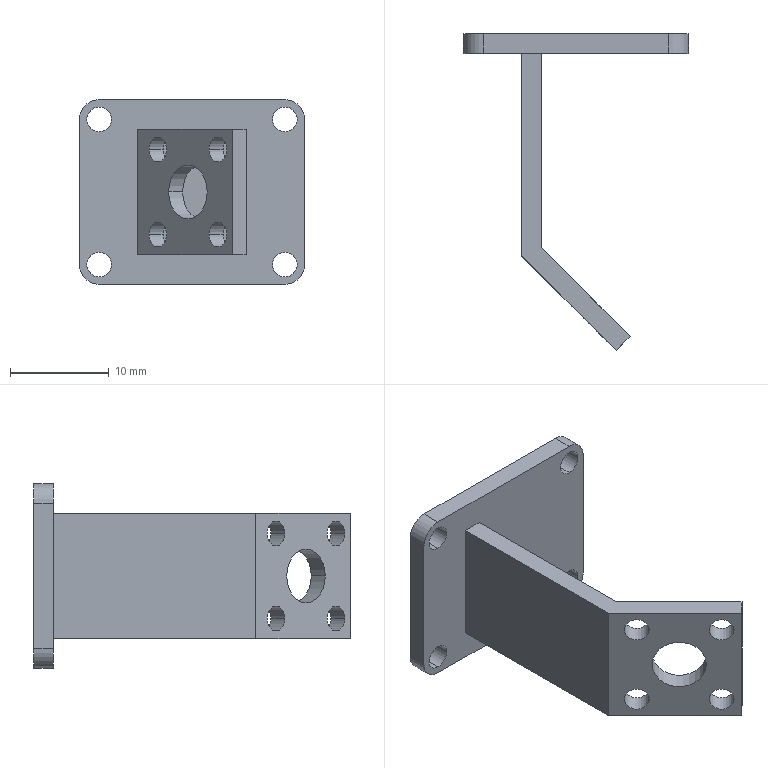Part | SolidWorks | features ICE 4, ExtruThin 1, Fillet 1 | 2 solids | 36 faces | box 22.8 x 32.073 x 18.7 mm | volume 1563 mm3 | cylinder 22 | plane 14 | commonest cylinder face diameters 2.5 x16 4 x4 5.5 x2
STEP:
#1=CARTESIAN_POINT('',(36.275,113.634,-14.95));
#2=VERTEX_POINT('',#1);
#3=CARTESIAN_POINT('',(36.275,113.634,-12.45));
#4=VERTEX_POINT('',#3);
#5=CARTESIAN_POINT('',(36.275,113.634,-13.7));
#6=DIRECTION('',(0.,1.,0.));
#7=DIRECTION('',(0.,0.,1.));
#8=AXIS2_PLACEMENT_3D('',#5,#6,#7);
#9=CIRCLE('',#8,1.25);
#10=EDGE_CURVE('',#2,#4,#9,.T.);
#11=ORIENTED_EDGE('',*,*,#10,.F.);
#12=CARTESIAN_POINT('',(36.275,115.634,-14.95));
#13=VERTEX_POINT('',#12);
#14=CARTESIAN_POINT('',(36.275,113.634,-14.95));
#15=DIRECTION('',(0.,1.,0.));
#16=VECTOR('',#15,1000.);
#17=LINE('',#14,#16);
#18=EDGE_CURVE('',#2,#13,#17,.T.);
#19=ORIENTED_EDGE('',*,*,#18,.T.);
#20=CARTESIAN_POINT('',(36.275,115.634,-12.45));
#21=VERTEX_POINT('',#20);
#22=CARTESIAN_POINT('',(36.275,115.634,-13.7));
#23=DIRECTION('',(0.,1.,0.));
#24=DIRECTION('',(0.,0.,1.));
#25=AXIS2_PLACEMENT_3D('',#22,#23,#24);
#26=CIRCLE('',#25,1.25);
#27=EDGE_CURVE('',#13,#21,#26,.T.);
#28=ORIENTED_EDGE('',*,*,#27,.T.);
#29=CARTESIAN_POINT('',(36.275,113.634,-12.45));
#30=DIRECTION('',(0.,1.,0.));
#31=VECTOR('',#30,1000.);
#32=LINE('',#29,#31);
#33=EDGE_CURVE('',#4,#21,#32,.T.);
#34=ORIENTED_EDGE('',*,*,#33,.F.);
#35=EDGE_LOOP('',(#11,#19,#28,#34));
#36=FACE_OUTER_BOUND('',#35,.T.);
#37=CARTESIAN_POINT('',(36.275,113.634,-13.7));
#38=DIRECTION('',(0.,1.,0.));
#39=DIRECTION('',(0.,0.,1.));
#40=AXIS2_PLACEMENT_3D('',#37,#38,#39);
#41=CYLINDRICAL_SURFACE('',#40,1.25);
#42=ADVANCED_FACE('',(#36),#41,.F.);
#43=CARTESIAN_POINT('',(36.275,113.634,-0.25));
#44=VERTEX_POINT('',#43);
#45=CARTESIAN_POINT('',(36.275,113.634,2.25));
#46=VERTEX_POINT('',#45);
#47=CARTESIAN_POINT('',(36.275,113.634,1.));
#48=DIRECTION('',(0.,1.,0.));
#49=DIRECTION('',(0.,0.,1.));
#50=AXIS2_PLACEMENT_3D('',#47,#48,#49);
#51=CIRCLE('',#50,1.25);
#52=EDGE_CURVE('',#44,#46,#51,.T.);
#53=ORIENTED_EDGE('',*,*,#52,.F.);
#54=CARTESIAN_POINT('',(36.275,115.634,-0.25));
#55=VERTEX_POINT('',#54);
#56=CARTESIAN_POINT('',(36.275,113.634,-0.25));
#57=DIRECTION('',(0.,1.,0.));
#58=VECTOR('',#57,1000.);
#59=LINE('',#56,#58);
#60=EDGE_CURVE('',#44,#55,#59,.T.);
#61=ORIENTED_EDGE('',*,*,#60,.T.);
#62=CARTESIAN_POINT('',(36.275,115.634,2.25));
#63=VERTEX_POINT('',#62);
#64=CARTESIAN_POINT('',(36.275,115.634,1.));
#65=DIRECTION('',(0.,1.,0.));
#66=DIRECTION('',(0.,0.,1.));
#67=AXIS2_PLACEMENT_3D('',#64,#65,#66);
#68=CIRCLE('',#67,1.25);
#69=EDGE_CURVE('',#55,#63,#68,.T.);
#70=ORIENTED_EDGE('',*,*,#69,.T.);
#71=CARTESIAN_POINT('',(36.275,113.634,2.25));
#72=DIRECTION('',(0.,1.,0.));
#73=VECTOR('',#72,1000.);
#74=LINE('',#71,#73);
#75=EDGE_CURVE('',#46,#63,#74,.T.);
#76=ORIENTED_EDGE('',*,*,#75,.F.);
#77=EDGE_LOOP('',(#53,#61,#70,#76));
#78=FACE_OUTER_BOUND('',#77,.T.);
#79=CARTESIAN_POINT('',(36.275,113.634,1.));
#80=DIRECTION('',(0.,1.,0.));
#81=DIRECTION('',(0.,0.,1.));
#82=AXIS2_PLACEMENT_3D('',#79,#80,#81);
#83=CYLINDRICAL_SURFACE('',#82,1.25);
#84=ADVANCED_FACE('',(#78),#83,.F.);
#85=CARTESIAN_POINT('',(55.075,113.634,-0.25));
#86=VERTEX_POINT('',#85);
#87=CARTESIAN_POINT('',(55.075,113.634,2.25));
#88=VERTEX_POINT('',#87);
#89=CARTESIAN_POINT('',(55.075,113.634,1.));
#90=DIRECTION('',(0.,1.,0.));
#91=DIRECTION('',(0.,0.,1.));
#92=AXIS2_PLACEMENT_3D('',#89,#90,#91);
#93=CIRCLE('',#92,1.25);
#94=EDGE_CURVE('',#86,#88,#93,.T.);
#95=ORIENTED_EDGE('',*,*,#94,.F.);
#96=CARTESIAN_POINT('',(55.075,115.634,-0.25));
#97=VERTEX_POINT('',#96);
#98=CARTESIAN_POINT('',(55.075,113.634,-0.25));
#99=DIRECTION('',(0.,1.,0.));
#100=VECTOR('',#99,1000.);
#101=LINE('',#98,#100);
#102=EDGE_CURVE('',#86,#97,#101,.T.);
#103=ORIENTED_EDGE('',*,*,#102,.T.);
#104=CARTESIAN_POINT('',(55.075,115.634,2.25));
#105=VERTEX_POINT('',#104);
#106=CARTESIAN_POINT('',(55.075,115.634,1.));
#107=DIRECTION('',(0.,1.,0.));
#108=DIRECTION('',(0.,0.,1.));
#109=AXIS2_PLACEMENT_3D('',#106,#107,#108);
#110=CIRCLE('',#109,1.25);
#111=EDGE_CURVE('',#97,#105,#110,.T.);
#112=ORIENTED_EDGE('',*,*,#111,.T.);
#113=CARTESIAN_POINT('',(55.075,113.634,2.25));
#114=DIRECTION('',(0.,1.,0.));
#115=VECTOR('',#114,1000.);
#116=LINE('',#113,#115);
#117=EDGE_CURVE('',#88,#105,#116,.T.);
#118=ORIENTED_EDGE('',*,*,#117,.F.);
#119=EDGE_LOOP('',(#95,#103,#112,#118));
#120=FACE_OUTER_BOUND('',#119,.T.);
#121=CARTESIAN_POINT('',(55.075,113.634,1.));
#122=DIRECTION('',(0.,1.,0.));
#123=DIRECTION('',(0.,0.,1.));
#124=AXIS2_PLACEMENT_3D('',#121,#122,#123);
#125=CYLINDRICAL_SURFACE('',#124,1.25);
#126=ADVANCED_FACE('',(#120),#125,.F.);
#127=CARTESIAN_POINT('',(55.075,113.634,-14.95));
#128=VERTEX_POINT('',#127);
#129=CARTESIAN_POINT('',(55.075,113.634,-12.45));
#130=VERTEX_POINT('',#129);
#131=CARTESIAN_POINT('',(55.075,113.634,-13.7));
#132=DIRECTION('',(0.,1.,0.));
#133=DIRECTION('',(0.,0.,1.));
#134=AXIS2_PLACEMENT_3D('',#131,#132,#133);
#135=CIRCLE('',#134,1.25);
#136=EDGE_CURVE('',#128,#130,#135,.T.);
#137=ORIENTED_EDGE('',*,*,#136,.F.);
#138=CARTESIAN_POINT('',(55.075,115.634,-14.95));
#139=VERTEX_POINT('',#138);
#140=CARTESIAN_POINT('',(55.075,113.634,-14.95));
#141=DIRECTION('',(0.,1.,0.));
#142=VECTOR('',#141,1000.);
#143=LINE('',#140,#142);
#144=EDGE_CURVE('',#128,#139,#143,.T.);
#145=ORIENTED_EDGE('',*,*,#144,.T.);
#146=CARTESIAN_POINT('',(55.075,115.634,-12.45));
#147=VERTEX_POINT('',#146);
#148=CARTESIAN_POINT('',(55.075,115.634,-13.7));
#149=DIRECTION('',(0.,1.,0.));
#150=DIRECTION('',(0.,0.,1.));
#151=AXIS2_PLACEMENT_3D('',#148,#149,#150);
#152=CIRCLE('',#151,1.25);
#153=EDGE_CURVE('',#139,#147,#152,.T.);
#154=ORIENTED_EDGE('',*,*,#153,.T.);
#155=CARTESIAN_POINT('',(55.075,113.634,-12.45));
#156=DIRECTION('',(0.,1.,0.));
#157=VECTOR('',#156,1000.);
#158=LINE('',#155,#157);
#159=EDGE_CURVE('',#130,#147,#158,.T.);
#160=ORIENTED_EDGE('',*,*,#159,.F.);
#161=EDGE_LOOP('',(#137,#145,#154,#160));
#162=FACE_OUTER_BOUND('',#161,.T.);
#163=CARTESIAN_POINT('',(55.075,113.634,-13.7));
#164=DIRECTION('',(0.,1.,0.));
#165=DIRECTION('',(0.,0.,1.));
#166=AXIS2_PLACEMENT_3D('',#163,#164,#165);
#167=CYLINDRICAL_SURFACE('',#166,1.25);
#168=ADVANCED_FACE('',(#162),#167,.F.);
#169=CARTESIAN_POINT('',(57.075,115.634,1.));
#170=VERTEX_POINT('',#169);
#171=CARTESIAN_POINT('',(57.075,115.634,-13.7));
#172=VERTEX_POINT('',#171);
#173=CARTESIAN_POINT('',(57.075,115.634,-15.7));
#174=DIRECTION('',(0.,0.,-1.));
#175=VECTOR('',#174,1000.);
#176=LINE('',#173,#175);
#177=EDGE_CURVE('',#170,#172,#176,.T.);
#178=ORIENTED_EDGE('',*,*,#177,.F.);
#179=CARTESIAN_POINT('',(57.075,113.634,1.));
#180=VERTEX_POINT('',#179);
#181=CARTESIAN_POINT('',(57.075,115.634,1.));
#182=DIRECTION('',(0.,-1.,0.));
#183=VECTOR('',#182,1000.);
#184=LINE('',#181,#183);
#185=EDGE_CURVE('',#170,#180,#184,.T.);
#186=ORIENTED_EDGE('',*,*,#185,.T.);
#187=CARTESIAN_POINT('',(57.075,113.634,-13.7));
#188=VERTEX_POINT('',#187);
#189=CARTESIAN_POINT('',(57.075,113.634,-15.7));
#190=DIRECTION('',(0.,0.,-1.));
#191=VECTOR('',#190,1000.);
#192=LINE('',#189,#191);
#193=EDGE_CURVE('',#180,#188,#192,.T.);
#194=ORIENTED_EDGE('',*,*,#193,.T.);
#195=CARTESIAN_POINT('',(57.075,115.634,-13.7));
#196=DIRECTION('',(0.,1.,0.));
#197=VECTOR('',#196,1000.);
#198=LINE('',#195,#197);
#199=EDGE_CURVE('',#188,#172,#198,.T.);
#200=ORIENTED_EDGE('',*,*,#199,.T.);
#201=EDGE_LOOP('',(#178,#186,#194,#200));
#202=FACE_OUTER_BOUND('',#201,.T.);
#203=CARTESIAN_POINT('',(57.075,115.634,-15.7));
#204=DIRECTION('',(-1.,0.,0.));
#205=DIRECTION('',(0.,0.,1.));
#206=AXIS2_PLACEMENT_3D('',#203,#204,#205);
#207=PLANE('',#206);
#208=ADVANCED_FACE('',(#202),#207,.F.);
#209=CARTESIAN_POINT('',(55.075,113.634,-15.7));
#210=VERTEX_POINT('',#209);
#211=CARTESIAN_POINT('',(36.275,113.634,-15.7));
#212=VERTEX_POINT('',#211);
#213=CARTESIAN_POINT('',(57.075,113.634,-15.7));
#214=DIRECTION('',(-1.,0.,0.));
#215=VECTOR('',#214,1000.);
#216=LINE('',#213,#215);
#217=EDGE_CURVE('',#210,#212,#216,.T.);
#218=ORIENTED_EDGE('',*,*,#217,.T.);
#219=CARTESIAN_POINT('',(36.275,115.634,-15.7));
#220=VERTEX_POINT('',#219);
#221=CARTESIAN_POINT('',(36.275,115.634,-15.7));
#222=DIRECTION('',(0.,1.,0.));
#223=VECTOR('',#222,1000.);
#224=LINE('',#221,#223);
#225=EDGE_CURVE('',#212,#220,#224,.T.);
#226=ORIENTED_EDGE('',*,*,#225,.T.);
#227=CARTESIAN_POINT('',(55.075,115.634,-15.7));
#228=VERTEX_POINT('',#227);
#229=CARTESIAN_POINT('',(57.075,115.634,-15.7));
#230=DIRECTION('',(-1.,0.,0.));
#231=VECTOR('',#230,1000.);
#232=LINE('',#229,#231);
#233=EDGE_CURVE('',#228,#220,#232,.T.);
#234=ORIENTED_EDGE('',*,*,#233,.F.);
#235=CARTESIAN_POINT('',(55.075,115.634,-15.7));
#236=DIRECTION('',(0.,-1.,0.));
#237=VECTOR('',#236,1000.);
#238=LINE('',#235,#237);
#239=EDGE_CURVE('',#228,#210,#238,.T.);
#240=ORIENTED_EDGE('',*,*,#239,.T.);
#241=EDGE_LOOP('',(#218,#226,#234,#240));
#242=FACE_OUTER_BOUND('',#241,.T.);
#243=CARTESIAN_POINT('',(57.075,115.634,-15.7));
#244=DIRECTION('',(0.,0.,1.));
#245=DIRECTION('',(1.,0.,0.));
#246=AXIS2_PLACEMENT_3D('',#243,#244,#245);
#247=PLANE('',#246);
#248=ADVANCED_FACE('',(#242),#247,.F.);
#249=CARTESIAN_POINT('',(34.275,113.634,-13.7));
#250=VERTEX_POINT('',#249);
#251=CARTESIAN_POINT('',(34.275,113.634,1.));
#252=VERTEX_POINT('',#251);
#253=CARTESIAN_POINT('',(34.275,113.634,-15.7));
#254=DIRECTION('',(0.,0.,1.));
#255=VECTOR('',#254,1000.);
#256=LINE('',#253,#255);
#257=EDGE_CURVE('',#250,#252,#256,.T.);
#258=ORIENTED_EDGE('',*,*,#257,.T.);
#259=CARTESIAN_POINT('',(34.275,115.634,1.));
#260=VERTEX_POINT('',#259);
#261=CARTESIAN_POINT('',(34.275,115.634,1.));
#262=DIRECTION('',(0.,1.,0.));
#263=VECTOR('',#262,1000.);
#264=LINE('',#261,#263);
#265=EDGE_CURVE('',#252,#260,#264,.T.);
#266=ORIENTED_EDGE('',*,*,#265,.T.);
#267=CARTESIAN_POINT('',(34.275,115.634,-13.7));
#268=VERTEX_POINT('',#267);
#269=CARTESIAN_POINT('',(34.275,115.634,-15.7));
#270=DIRECTION('',(0.,0.,1.));
#271=VECTOR('',#270,1000.);
#272=LINE('',#269,#271);
#273=EDGE_CURVE('',#268,#260,#272,.T.);
#274=ORIENTED_EDGE('',*,*,#273,.F.);
#275=CARTESIAN_POINT('',(34.275,115.634,-13.7));
#276=DIRECTION('',(0.,-1.,0.));
#277=VECTOR('',#276,1000.);
#278=LINE('',#275,#277);
#279=EDGE_CURVE('',#268,#250,#278,.T.);
#280=ORIENTED_EDGE('',*,*,#279,.T.);
#281=EDGE_LOOP('',(#258,#266,#274,#280));
#282=FACE_OUTER_BOUND('',#281,.T.);
#283=CARTESIAN_POINT('',(34.275,115.634,-15.7));
#284=DIRECTION('',(1.,0.,0.));
#285=DIRECTION('',(0.,0.,-1.));
#286=AXIS2_PLACEMENT_3D('',#283,#284,#285);
#287=PLANE('',#286);
#288=ADVANCED_FACE('',(#282),#287,.F.);
#289=CARTESIAN_POINT('',(36.275,113.634,3.));
#290=VERTEX_POINT('',#289);
#291=CARTESIAN_POINT('',(55.075,113.634,3.));
#292=VERTEX_POINT('',#291);
#293=CARTESIAN_POINT('',(57.075,113.634,3.));
#294=DIRECTION('',(1.,0.,0.));
#295=VECTOR('',#294,1000.);
#296=LINE('',#293,#295);
#297=EDGE_CURVE('',#290,#292,#296,.T.);
#298=ORIENTED_EDGE('',*,*,#297,.T.);
#299=CARTESIAN_POINT('',(55.075,115.634,3.));
#300=VERTEX_POINT('',#299);
#301=CARTESIAN_POINT('',(55.075,115.634,3.));
#302=DIRECTION('',(0.,1.,0.));
#303=VECTOR('',#302,1000.);
#304=LINE('',#301,#303);
#305=EDGE_CURVE('',#292,#300,#304,.T.);
#306=ORIENTED_EDGE('',*,*,#305,.T.);
#307=CARTESIAN_POINT('',(36.275,115.634,3.));
#308=VERTEX_POINT('',#307);
#309=CARTESIAN_POINT('',(57.075,115.634,3.));
#310=DIRECTION('',(1.,0.,0.));
#311=VECTOR('',#310,1000.);
#312=LINE('',#309,#311);
#313=EDGE_CURVE('',#308,#300,#312,.T.);
#314=ORIENTED_EDGE('',*,*,#313,.F.);
#315=CARTESIAN_POINT('',(36.275,115.634,3.));
#316=DIRECTION('',(0.,-1.,0.));
#317=VECTOR('',#316,1000.);
#318=LINE('',#315,#317);
#319=EDGE_CURVE('',#308,#290,#318,.T.);
#320=ORIENTED_EDGE('',*,*,#319,.T.);
#321=EDGE_LOOP('',(#298,#306,#314,#320));
#322=FACE_OUTER_BOUND('',#321,.T.);
#323=CARTESIAN_POINT('',(57.075,115.634,3.));
#324=DIRECTION('',(0.,0.,-1.));
#325=DIRECTION('',(-1.,0.,0.));
#326=AXIS2_PLACEMENT_3D('',#323,#324,#325);
#327=PLANE('',#326);
#328=ADVANCED_FACE('',(#322),#327,.F.);
#329=CARTESIAN_POINT('',(36.275,115.634,-13.7));
#330=DIRECTION('',(0.,1.,0.));
#331=DIRECTION('',(0.,0.,1.));
#332=AXIS2_PLACEMENT_3D('',#329,#330,#331);
#333=CIRCLE('',#332,1.25);
#334=EDGE_CURVE('',#21,#13,#333,.T.);
#335=ORIENTED_EDGE('',*,*,#334,.F.);
#336=ORIENTED_EDGE('',*,*,#27,.F.);
#337=EDGE_LOOP('',(#335,#336));
#338=FACE_BOUND('',#337,.T.);
#339=CARTESIAN_POINT('',(36.275,115.634,1.));
#340=DIRECTION('',(0.,1.,0.));
#341=DIRECTION('',(0.,0.,1.));
#342=AXIS2_PLACEMENT_3D('',#339,#340,#341);
#343=CIRCLE('',#342,1.25);
#344=EDGE_CURVE('',#63,#55,#343,.T.);
#345=ORIENTED_EDGE('',*,*,#344,.F.);
#346=ORIENTED_EDGE('',*,*,#69,.F.);
#347=EDGE_LOOP('',(#345,#346));
#348=FACE_BOUND('',#347,.T.);
#349=CARTESIAN_POINT('',(55.075,115.634,1.));
#350=DIRECTION('',(0.,1.,0.));
#351=DIRECTION('',(0.,0.,1.));
#352=AXIS2_PLACEMENT_3D('',#349,#350,#351);
#353=CIRCLE('',#352,1.25);
#354=EDGE_CURVE('',#105,#97,#353,.T.);
#355=ORIENTED_EDGE('',*,*,#354,.F.);
#356=ORIENTED_EDGE('',*,*,#111,.F.);
#357=EDGE_LOOP('',(#355,#356));
#358=FACE_BOUND('',#357,.T.);
#359=CARTESIAN_POINT('',(55.075,115.634,-13.7));
#360=DIRECTION('',(0.,1.,0.));
#361=DIRECTION('',(0.,0.,1.));
#362=AXIS2_PLACEMENT_3D('',#359,#360,#361);
#363=CIRCLE('',#362,1.25);
#364=EDGE_CURVE('',#147,#139,#363,.T.);
#365=ORIENTED_EDGE('',*,*,#364,.F.);
#366=ORIENTED_EDGE('',*,*,#153,.F.);
#367=EDGE_LOOP('',(#365,#366));
#368=FACE_BOUND('',#367,.T.);
#369=ORIENTED_EDGE('',*,*,#313,.T.);
#370=CARTESIAN_POINT('',(55.075,115.634,1.));
#371=DIRECTION('',(0.,1.,0.));
#372=DIRECTION('',(0.,0.,-1.));
#373=AXIS2_PLACEMENT_3D('',#370,#371,#372);
#374=CIRCLE('',#373,2.);
#375=EDGE_CURVE('',#300,#170,#374,.T.);
#376=ORIENTED_EDGE('',*,*,#375,.T.);
#377=ORIENTED_EDGE('',*,*,#177,.T.);
#378=CARTESIAN_POINT('',(55.075,115.634,-13.7));
#379=DIRECTION('',(0.,1.,0.));
#380=DIRECTION('',(0.,0.,-1.));
#381=AXIS2_PLACEMENT_3D('',#378,#379,#380);
#382=CIRCLE('',#381,2.);
#383=EDGE_CURVE('',#172,#228,#382,.T.);
#384=ORIENTED_EDGE('',*,*,#383,.T.);
#385=ORIENTED_EDGE('',*,*,#233,.T.);
#386=CARTESIAN_POINT('',(36.275,115.634,-13.7));
#387=DIRECTION('',(0.,1.,0.));
#388=DIRECTION('',(0.,0.,-1.));
#389=AXIS2_PLACEMENT_3D('',#386,#387,#388);
#390=CIRCLE('',#389,2.);
#391=EDGE_CURVE('',#220,#268,#390,.T.);
#392=ORIENTED_EDGE('',*,*,#391,.T.);
#393=ORIENTED_EDGE('',*,*,#273,.T.);
#394=CARTESIAN_POINT('',(36.275,115.634,1.));
#395=DIRECTION('',(0.,1.,0.));
#396=DIRECTION('',(0.,0.,-1.));
#397=AXIS2_PLACEMENT_3D('',#394,#395,#396);
#398=CIRCLE('',#397,2.);
#399=EDGE_CURVE('',#260,#308,#398,.T.);
#400=ORIENTED_EDGE('',*,*,#399,.T.);
#401=EDGE_LOOP('',(#369,#376,#377,#384,#385,#392,#393,#400));
#402=FACE_OUTER_BOUND('',#401,.T.);
#403=CARTESIAN_POINT('',(0.,115.634,0.));
#404=DIRECTION('',(0.,-1.,0.));
#405=DIRECTION('',(0.,0.,-1.));
#406=AXIS2_PLACEMENT_3D('',#403,#404,#405);
#407=PLANE('',#406);
#408=ADVANCED_FACE('',(#338,#348,#358,#368,#402),#407,.F.);
#409=CARTESIAN_POINT('',(36.275,113.634,-13.7));
#410=DIRECTION('',(0.,1.,0.));
#411=DIRECTION('',(0.,0.,1.));
#412=AXIS2_PLACEMENT_3D('',#409,#410,#411);
#413=CIRCLE('',#412,1.25);
#414=EDGE_CURVE('',#4,#2,#413,.T.);
#415=ORIENTED_EDGE('',*,*,#414,.T.);
#416=ORIENTED_EDGE('',*,*,#10,.T.);
#417=EDGE_LOOP('',(#415,#416));
#418=FACE_BOUND('',#417,.T.);
#419=CARTESIAN_POINT('',(36.275,113.634,1.));
#420=DIRECTION('',(0.,1.,0.));
#421=DIRECTION('',(0.,0.,1.));
#422=AXIS2_PLACEMENT_3D('',#419,#420,#421);
#423=CIRCLE('',#422,1.25);
#424=EDGE_CURVE('',#46,#44,#423,.T.);
#425=ORIENTED_EDGE('',*,*,#424,.T.);
#426=ORIENTED_EDGE('',*,*,#52,.T.);
#427=EDGE_LOOP('',(#425,#426));
#428=FACE_BOUND('',#427,.T.);
#429=CARTESIAN_POINT('',(55.075,113.634,1.));
#430=DIRECTION('',(0.,1.,0.));
#431=DIRECTION('',(0.,0.,1.));
#432=AXIS2_PLACEMENT_3D('',#429,#430,#431);
#433=CIRCLE('',#432,1.25);
#434=EDGE_CURVE('',#88,#86,#433,.T.);
#435=ORIENTED_EDGE('',*,*,#434,.T.);
#436=ORIENTED_EDGE('',*,*,#94,.T.);
#437=EDGE_LOOP('',(#435,#436));
#438=FACE_BOUND('',#437,.T.);
#439=CARTESIAN_POINT('',(55.075,113.634,-13.7));
#440=DIRECTION('',(0.,1.,0.));
#441=DIRECTION('',(0.,0.,1.));
#442=AXIS2_PLACEMENT_3D('',#439,#440,#441);
#443=CIRCLE('',#442,1.25);
#444=EDGE_CURVE('',#130,#128,#443,.T.);
#445=ORIENTED_EDGE('',*,*,#444,.T.);
#446=ORIENTED_EDGE('',*,*,#136,.T.);
#447=EDGE_LOOP('',(#445,#446));
#448=FACE_BOUND('',#447,.T.);
#449=ORIENTED_EDGE('',*,*,#193,.F.);
#450=CARTESIAN_POINT('',(55.075,113.634,1.));
#451=DIRECTION('',(0.,-1.,0.));
#452=DIRECTION('',(0.,0.,-1.));
#453=AXIS2_PLACEMENT_3D('',#450,#451,#452);
#454=CIRCLE('',#453,2.);
#455=EDGE_CURVE('',#180,#292,#454,.T.);
#456=ORIENTED_EDGE('',*,*,#455,.T.);
#457=ORIENTED_EDGE('',*,*,#297,.F.);
#458=CARTESIAN_POINT('',(36.275,113.634,1.));
#459=DIRECTION('',(0.,-1.,0.));
#460=DIRECTION('',(0.,0.,-1.));
#461=AXIS2_PLACEMENT_3D('',#458,#459,#460);
#462=CIRCLE('',#461,2.);
#463=EDGE_CURVE('',#290,#252,#462,.T.);
#464=ORIENTED_EDGE('',*,*,#463,.T.);
#465=ORIENTED_EDGE('',*,*,#257,.F.);
#466=CARTESIAN_POINT('',(36.275,113.634,-13.7));
#467=DIRECTION('',(0.,-1.,0.));
#468=DIRECTION('',(0.,0.,-1.));
#469=AXIS2_PLACEMENT_3D('',#466,#467,#468);
#470=CIRCLE('',#469,2.);
#471=EDGE_CURVE('',#250,#212,#470,.T.);
#472=ORIENTED_EDGE('',*,*,#471,.T.);
#473=ORIENTED_EDGE('',*,*,#217,.F.);
#474=CARTESIAN_POINT('',(55.075,113.634,-13.7));
#475=DIRECTION('',(0.,-1.,0.));
#476=DIRECTION('',(0.,0.,-1.));
#477=AXIS2_PLACEMENT_3D('',#474,#475,#476);
#478=CIRCLE('',#477,2.);
#479=EDGE_CURVE('',#210,#188,#478,.T.);
#480=ORIENTED_EDGE('',*,*,#479,.T.);
#481=EDGE_LOOP('',(#449,#456,#457,#464,#465,#472,#473,#480));
#482=FACE_OUTER_BOUND('',#481,.T.);
#483=CARTESIAN_POINT('',(0.,113.634,0.));
#484=DIRECTION('',(0.,-1.,0.));
#485=DIRECTION('',(0.,0.,-1.));
#486=AXIS2_PLACEMENT_3D('',#483,#484,#485);
#487=PLANE('',#486);
#488=ADVANCED_FACE('',(#418,#428,#438,#448,#482),#487,.T.);
#489=ORIENTED_EDGE('',*,*,#375,.F.);
#490=ORIENTED_EDGE('',*,*,#305,.F.);
#491=ORIENTED_EDGE('',*,*,#455,.F.);
#492=ORIENTED_EDGE('',*,*,#185,.F.);
#493=EDGE_LOOP('',(#489,#490,#491,#492));
#494=FACE_OUTER_BOUND('',#493,.T.);
#495=CARTESIAN_POINT('',(55.075,115.634,1.));
#496=DIRECTION('',(0.,-1.,0.));
#497=DIRECTION('',(0.,0.,-1.));
#498=AXIS2_PLACEMENT_3D('',#495,#496,#497);
#499=CYLINDRICAL_SURFACE('',#498,2.);
#500=ADVANCED_FACE('',(#494),#499,.T.);
#501=ORIENTED_EDGE('',*,*,#399,.F.);
#502=ORIENTED_EDGE('',*,*,#265,.F.);
#503=ORIENTED_EDGE('',*,*,#463,.F.);
#504=ORIENTED_EDGE('',*,*,#319,.F.);
#505=EDGE_LOOP('',(#501,#502,#503,#504));
#506=FACE_OUTER_BOUND('',#505,.T.);
#507=CARTESIAN_POINT('',(36.275,115.634,1.));
#508=DIRECTION('',(0.,-1.,0.));
#509=DIRECTION('',(0.,0.,-1.));
#510=AXIS2_PLACEMENT_3D('',#507,#508,#509);
#511=CYLINDRICAL_SURFACE('',#510,2.);
#512=ADVANCED_FACE('',(#506),#511,.T.);
#513=ORIENTED_EDGE('',*,*,#391,.F.);
#514=ORIENTED_EDGE('',*,*,#225,.F.);
#515=ORIENTED_EDGE('',*,*,#471,.F.);
#516=ORIENTED_EDGE('',*,*,#279,.F.);
#517=EDGE_LOOP('',(#513,#514,#515,#516));
#518=FACE_OUTER_BOUND('',#517,.T.);
#519=CARTESIAN_POINT('',(36.275,115.634,-13.7));
#520=DIRECTION('',(0.,-1.,0.));
#521=DIRECTION('',(0.,0.,-1.));
#522=AXIS2_PLACEMENT_3D('',#519,#520,#521);
#523=CYLINDRICAL_SURFACE('',#522,2.);
#524=ADVANCED_FACE('',(#518),#523,.T.);
#525=ORIENTED_EDGE('',*,*,#383,.F.);
#526=ORIENTED_EDGE('',*,*,#199,.F.);
#527=ORIENTED_EDGE('',*,*,#479,.F.);
#528=ORIENTED_EDGE('',*,*,#239,.F.);
#529=EDGE_LOOP('',(#525,#526,#527,#528));
#530=FACE_OUTER_BOUND('',#529,.T.);
#531=CARTESIAN_POINT('',(55.075,115.634,-13.7));
#532=DIRECTION('',(0.,-1.,0.));
#533=DIRECTION('',(0.,0.,-1.));
#534=AXIS2_PLACEMENT_3D('',#531,#532,#533);
#535=CYLINDRICAL_SURFACE('',#534,2.);
#536=ADVANCED_FACE('',(#530),#535,.T.);
#537=ORIENTED_EDGE('',*,*,#144,.F.);
#538=ORIENTED_EDGE('',*,*,#444,.F.);
#539=ORIENTED_EDGE('',*,*,#159,.T.);
#540=ORIENTED_EDGE('',*,*,#364,.T.);
#541=EDGE_LOOP('',(#537,#538,#539,#540));
#542=FACE_OUTER_BOUND('',#541,.T.);
#543=CARTESIAN_POINT('',(55.075,113.634,-13.7));
#544=DIRECTION('',(0.,1.,0.));
#545=DIRECTION('',(0.,0.,1.));
#546=AXIS2_PLACEMENT_3D('',#543,#544,#545);
#547=CYLINDRICAL_SURFACE('',#546,1.25);
#548=ADVANCED_FACE('',(#542),#547,.F.);
#549=ORIENTED_EDGE('',*,*,#102,.F.);
#550=ORIENTED_EDGE('',*,*,#434,.F.);
#551=ORIENTED_EDGE('',*,*,#117,.T.);
#552=ORIENTED_EDGE('',*,*,#354,.T.);
#553=EDGE_LOOP('',(#549,#550,#551,#552));
#554=FACE_OUTER_BOUND('',#553,.T.);
#555=CARTESIAN_POINT('',(55.075,113.634,1.));
#556=DIRECTION('',(0.,1.,0.));
#557=DIRECTION('',(0.,0.,1.));
#558=AXIS2_PLACEMENT_3D('',#555,#556,#557);
#559=CYLINDRICAL_SURFACE('',#558,1.25);
#560=ADVANCED_FACE('',(#554),#559,.F.);
#561=ORIENTED_EDGE('',*,*,#60,.F.);
#562=ORIENTED_EDGE('',*,*,#424,.F.);
#563=ORIENTED_EDGE('',*,*,#75,.T.);
#564=ORIENTED_EDGE('',*,*,#344,.T.);
#565=EDGE_LOOP('',(#561,#562,#563,#564));
#566=FACE_OUTER_BOUND('',#565,.T.);
#567=CARTESIAN_POINT('',(36.275,113.634,1.));
#568=DIRECTION('',(0.,1.,0.));
#569=DIRECTION('',(0.,0.,1.));
#570=AXIS2_PLACEMENT_3D('',#567,#568,#569);
#571=CYLINDRICAL_SURFACE('',#570,1.25);
#572=ADVANCED_FACE('',(#566),#571,.F.);
#573=ORIENTED_EDGE('',*,*,#18,.F.);
#574=ORIENTED_EDGE('',*,*,#414,.F.);
#575=ORIENTED_EDGE('',*,*,#33,.T.);
#576=ORIENTED_EDGE('',*,*,#334,.T.);
#577=EDGE_LOOP('',(#573,#574,#575,#576));
#578=FACE_OUTER_BOUND('',#577,.T.);
#579=CARTESIAN_POINT('',(36.275,113.634,-13.7));
#580=DIRECTION('',(0.,1.,0.));
#581=DIRECTION('',(0.,0.,1.));
#582=AXIS2_PLACEMENT_3D('',#579,#580,#581);
#583=CYLINDRICAL_SURFACE('',#582,1.25);
#584=ADVANCED_FACE('',(#578),#583,.F.);
#585=CLOSED_SHELL('',(#42,#84,#126,#168,#208,#248,#288,#328,#408,#488,#500,#512,#524,#536,#548,#560,#572,#584));
#586=MANIFOLD_SOLID_BREP('',#585);
#587=CARTESIAN_POINT('',(50.6,85.541,-10.65));
#588=VERTEX_POINT('',#587);
#589=CARTESIAN_POINT('',(48.832,87.309,-10.65));
#590=VERTEX_POINT('',#589);
#591=CARTESIAN_POINT('',(49.716,86.425,-10.65));
#592=DIRECTION('',(0.7071,0.7071,0.));
#593=DIRECTION('',(-0.7071,0.7071,0.));
#594=AXIS2_PLACEMENT_3D('',#591,#592,#593);
#595=CIRCLE('',#594,1.25);
#596=EDGE_CURVE('',#588,#590,#595,.T.);
#597=ORIENTED_EDGE('',*,*,#596,.T.);
#598=CARTESIAN_POINT('',(47.418,85.895,-10.65));
#599=VERTEX_POINT('',#598);
#600=CARTESIAN_POINT('',(54.489,92.966,-10.65));
#601=DIRECTION('',(-0.7071,-0.7071,0.));
#602=VECTOR('',#601,1000.);
#603=LINE('',#600,#602);
#604=EDGE_CURVE('',#590,#599,#603,.T.);
#605=ORIENTED_EDGE('',*,*,#604,.T.);
#606=CARTESIAN_POINT('',(49.186,84.127,-10.65));
#607=VERTEX_POINT('',#606);
#608=CARTESIAN_POINT('',(48.302,85.011,-10.65));
#609=DIRECTION('',(-0.7071,-0.7071,0.));
#610=DIRECTION('',(0.7071,-0.7071,0.));
#611=AXIS2_PLACEMENT_3D('',#608,#609,#610);
#612=CIRCLE('',#611,1.25);
#613=EDGE_CURVE('',#599,#607,#612,.T.);
#614=ORIENTED_EDGE('',*,*,#613,.T.);
#615=CARTESIAN_POINT('',(56.257,91.198,-10.65));
#616=DIRECTION('',(-0.7071,-0.7071,0.));
#617=VECTOR('',#616,1000.);
#618=LINE('',#615,#617);
#619=EDGE_CURVE('',#588,#607,#618,.T.);
#620=ORIENTED_EDGE('',*,*,#619,.F.);
#621=EDGE_LOOP('',(#597,#605,#614,#620));
#622=FACE_OUTER_BOUND('',#621,.T.);
#623=CARTESIAN_POINT('',(55.373,92.082,-10.65));
#624=DIRECTION('',(-0.7071,-0.7071,0.));
#625=DIRECTION('',(0.7071,-0.7071,0.));
#626=AXIS2_PLACEMENT_3D('',#623,#624,#625);
#627=CYLINDRICAL_SURFACE('',#626,1.25);
#628=ADVANCED_FACE('',(#622),#627,.F.);
#629=CARTESIAN_POINT('',(44.519,91.622,-2.05));
#630=VERTEX_POINT('',#629);
#631=CARTESIAN_POINT('',(42.751,93.39,-2.05));
#632=VERTEX_POINT('',#631);
#633=CARTESIAN_POINT('',(43.635,92.506,-2.05));
#634=DIRECTION('',(0.7071,0.7071,0.));
#635=DIRECTION('',(-0.7071,0.7071,0.));
#636=AXIS2_PLACEMENT_3D('',#633,#634,#635);
#637=CIRCLE('',#636,1.25);
#638=EDGE_CURVE('',#630,#632,#637,.T.);
#639=ORIENTED_EDGE('',*,*,#638,.T.);
#640=CARTESIAN_POINT('',(41.337,91.976,-2.05));
#641=VERTEX_POINT('',#640);
#642=CARTESIAN_POINT('',(48.408,99.047,-2.05));
#643=DIRECTION('',(-0.7071,-0.7071,0.));
#644=VECTOR('',#643,1000.);
#645=LINE('',#642,#644);
#646=EDGE_CURVE('',#632,#641,#645,.T.);
#647=ORIENTED_EDGE('',*,*,#646,.T.);
#648=CARTESIAN_POINT('',(43.105,90.208,-2.05));
#649=VERTEX_POINT('',#648);
#650=CARTESIAN_POINT('',(42.221,91.092,-2.05));
#651=DIRECTION('',(-0.7071,-0.7071,0.));
#652=DIRECTION('',(0.7071,-0.7071,0.));
#653=AXIS2_PLACEMENT_3D('',#650,#651,#652);
#654=CIRCLE('',#653,1.25);
#655=EDGE_CURVE('',#641,#649,#654,.T.);
#656=ORIENTED_EDGE('',*,*,#655,.T.);
#657=CARTESIAN_POINT('',(50.176,97.279,-2.05));
#658=DIRECTION('',(-0.7071,-0.7071,0.));
#659=VECTOR('',#658,1000.);
#660=LINE('',#657,#659);
#661=EDGE_CURVE('',#630,#649,#660,.T.);
#662=ORIENTED_EDGE('',*,*,#661,.F.);
#663=EDGE_LOOP('',(#639,#647,#656,#662));
#664=FACE_OUTER_BOUND('',#663,.T.);
#665=CARTESIAN_POINT('',(49.292,98.163,-2.05));
#666=DIRECTION('',(-0.7071,-0.7071,0.));
#667=DIRECTION('',(0.7071,-0.7071,0.));
#668=AXIS2_PLACEMENT_3D('',#665,#666,#667);
#669=CYLINDRICAL_SURFACE('',#668,1.25);
#670=ADVANCED_FACE('',(#664),#669,.F.);
#671=CARTESIAN_POINT('',(50.6,85.541,-2.05));
#672=VERTEX_POINT('',#671);
#673=CARTESIAN_POINT('',(48.832,87.309,-2.05));
#674=VERTEX_POINT('',#673);
#675=CARTESIAN_POINT('',(49.716,86.425,-2.05));
#676=DIRECTION('',(0.7071,0.7071,0.));
#677=DIRECTION('',(-0.7071,0.7071,0.));
#678=AXIS2_PLACEMENT_3D('',#675,#676,#677);
#679=CIRCLE('',#678,1.25);
#680=EDGE_CURVE('',#672,#674,#679,.T.);
#681=ORIENTED_EDGE('',*,*,#680,.T.);
#682=CARTESIAN_POINT('',(47.418,85.895,-2.05));
#683=VERTEX_POINT('',#682);
#684=CARTESIAN_POINT('',(54.489,92.966,-2.05));
#685=DIRECTION('',(-0.7071,-0.7071,0.));
#686=VECTOR('',#685,1000.);
#687=LINE('',#684,#686);
#688=EDGE_CURVE('',#674,#683,#687,.T.);
#689=ORIENTED_EDGE('',*,*,#688,.T.);
#690=CARTESIAN_POINT('',(49.186,84.127,-2.05));
#691=VERTEX_POINT('',#690);
#692=CARTESIAN_POINT('',(48.302,85.011,-2.05));
#693=DIRECTION('',(-0.7071,-0.7071,0.));
#694=DIRECTION('',(0.7071,-0.7071,0.));
#695=AXIS2_PLACEMENT_3D('',#692,#693,#694);
#696=CIRCLE('',#695,1.25);
#697=EDGE_CURVE('',#683,#691,#696,.T.);
#698=ORIENTED_EDGE('',*,*,#697,.T.);
#699=CARTESIAN_POINT('',(56.257,91.198,-2.05));
#700=DIRECTION('',(-0.7071,-0.7071,0.));
#701=VECTOR('',#700,1000.);
#702=LINE('',#699,#701);
#703=EDGE_CURVE('',#672,#691,#702,.T.);
#704=ORIENTED_EDGE('',*,*,#703,.F.);
#705=EDGE_LOOP('',(#681,#689,#698,#704));
#706=FACE_OUTER_BOUND('',#705,.T.);
#707=CARTESIAN_POINT('',(55.373,92.082,-2.05));
#708=DIRECTION('',(-0.7071,-0.7071,0.));
#709=DIRECTION('',(0.7071,-0.7071,0.));
#710=AXIS2_PLACEMENT_3D('',#707,#708,#709);
#711=CYLINDRICAL_SURFACE('',#710,1.25);
#712=ADVANCED_FACE('',(#706),#711,.F.);
#713=CARTESIAN_POINT('',(44.519,91.622,-10.65));
#714=VERTEX_POINT('',#713);
#715=CARTESIAN_POINT('',(42.751,93.39,-10.65));
#716=VERTEX_POINT('',#715);
#717=CARTESIAN_POINT('',(43.635,92.506,-10.65));
#718=DIRECTION('',(0.7071,0.7071,0.));
#719=DIRECTION('',(-0.7071,0.7071,0.));
#720=AXIS2_PLACEMENT_3D('',#717,#718,#719);
#721=CIRCLE('',#720,1.25);
#722=EDGE_CURVE('',#714,#716,#721,.T.);
#723=ORIENTED_EDGE('',*,*,#722,.T.);
#724=CARTESIAN_POINT('',(41.337,91.976,-10.65));
#725=VERTEX_POINT('',#724);
#726=CARTESIAN_POINT('',(48.408,99.047,-10.65));
#727=DIRECTION('',(-0.7071,-0.7071,0.));
#728=VECTOR('',#727,1000.);
#729=LINE('',#726,#728);
#730=EDGE_CURVE('',#716,#725,#729,.T.);
#731=ORIENTED_EDGE('',*,*,#730,.T.);
#732=CARTESIAN_POINT('',(43.105,90.208,-10.65));
#733=VERTEX_POINT('',#732);
#734=CARTESIAN_POINT('',(42.221,91.092,-10.65));
#735=DIRECTION('',(-0.7071,-0.7071,0.));
#736=DIRECTION('',(0.7071,-0.7071,0.));
#737=AXIS2_PLACEMENT_3D('',#734,#735,#736);
#738=CIRCLE('',#737,1.25);
#739=EDGE_CURVE('',#725,#733,#738,.T.);
#740=ORIENTED_EDGE('',*,*,#739,.T.);
#741=CARTESIAN_POINT('',(50.176,97.279,-10.65));
#742=DIRECTION('',(-0.7071,-0.7071,0.));
#743=VECTOR('',#742,1000.);
#744=LINE('',#741,#743);
#745=EDGE_CURVE('',#714,#733,#744,.T.);
#746=ORIENTED_EDGE('',*,*,#745,.F.);
#747=EDGE_LOOP('',(#723,#731,#740,#746));
#748=FACE_OUTER_BOUND('',#747,.T.);
#749=CARTESIAN_POINT('',(49.292,98.163,-10.65));
#750=DIRECTION('',(-0.7071,-0.7071,0.));
#751=DIRECTION('',(0.7071,-0.7071,0.));
#752=AXIS2_PLACEMENT_3D('',#749,#750,#751);
#753=CYLINDRICAL_SURFACE('',#752,1.25);
#754=ADVANCED_FACE('',(#748),#753,.F.);
#755=CARTESIAN_POINT('',(47.206,86.107,-6.35));
#756=VERTEX_POINT('',#755);
#757=CARTESIAN_POINT('',(43.317,89.996,-6.35));
#758=VERTEX_POINT('',#757);
#759=CARTESIAN_POINT('',(45.261,88.052,-6.35));
#760=DIRECTION('',(0.7071,0.7071,0.));
#761=DIRECTION('',(-0.7071,0.7071,0.));
#762=AXIS2_PLACEMENT_3D('',#759,#760,#761);
#763=CIRCLE('',#762,2.75);
#764=EDGE_CURVE('',#756,#758,#763,.T.);
#765=ORIENTED_EDGE('',*,*,#764,.F.);
#766=CARTESIAN_POINT('',(48.62,87.521,-6.35));
#767=VERTEX_POINT('',#766);
#768=CARTESIAN_POINT('',(39.468,78.369,-6.35));
#769=DIRECTION('',(0.7071,0.7071,0.));
#770=VECTOR('',#769,1000.);
#771=LINE('',#768,#770);
#772=EDGE_CURVE('',#756,#767,#771,.T.);
#773=ORIENTED_EDGE('',*,*,#772,.T.);
#774=CARTESIAN_POINT('',(44.731,91.41,-6.35));
#775=VERTEX_POINT('',#774);
#776=CARTESIAN_POINT('',(46.675,89.466,-6.35));
#777=DIRECTION('',(0.7071,0.7071,0.));
#778=DIRECTION('',(-0.7071,0.7071,0.));
#779=AXIS2_PLACEMENT_3D('',#776,#777,#778);
#780=CIRCLE('',#779,2.75);
#781=EDGE_CURVE('',#767,#775,#780,.T.);
#782=ORIENTED_EDGE('',*,*,#781,.T.);
#783=CARTESIAN_POINT('',(35.579,82.258,-6.35));
#784=DIRECTION('',(0.7071,0.7071,0.));
#785=VECTOR('',#784,1000.);
#786=LINE('',#783,#785);
#787=EDGE_CURVE('',#758,#775,#786,.T.);
#788=ORIENTED_EDGE('',*,*,#787,.F.);
#789=EDGE_LOOP('',(#765,#773,#782,#788));
#790=FACE_OUTER_BOUND('',#789,.T.);
#791=CARTESIAN_POINT('',(37.523,80.314,-6.35));
#792=DIRECTION('',(0.7071,0.7071,0.));
#793=DIRECTION('',(-0.7071,0.7071,0.));
#794=AXIS2_PLACEMENT_3D('',#791,#792,#793);
#795=CYLINDRICAL_SURFACE('',#794,2.75);
#796=ADVANCED_FACE('',(#790),#795,.F.);
#797=CARTESIAN_POINT('',(42.185,93.956,0.));
#798=VERTEX_POINT('',#797);
#799=CARTESIAN_POINT('',(42.185,113.634,0.));
#800=VERTEX_POINT('',#799);
#801=CARTESIAN_POINT('',(42.185,93.956,0.));
#802=DIRECTION('',(0.,1.,0.));
#803=VECTOR('',#802,1000.);
#804=LINE('',#801,#803);
#805=EDGE_CURVE('',#798,#800,#804,.T.);
#806=ORIENTED_EDGE('',*,*,#805,.F.);
#807=CARTESIAN_POINT('',(42.185,93.956,-12.7));
#808=VERTEX_POINT('',#807);
#809=CARTESIAN_POINT('',(42.185,93.956,-12.7));
#810=DIRECTION('',(0.,0.,1.));
#811=VECTOR('',#810,1000.);
#812=LINE('',#809,#811);
#813=EDGE_CURVE('',#808,#798,#812,.T.);
#814=ORIENTED_EDGE('',*,*,#813,.F.);
#815=CARTESIAN_POINT('',(42.185,113.634,-12.7));
#816=VERTEX_POINT('',#815);
#817=CARTESIAN_POINT('',(42.185,93.956,-12.7));
#818=DIRECTION('',(0.,1.,0.));
#819=VECTOR('',#818,1000.);
#820=LINE('',#817,#819);
#821=EDGE_CURVE('',#808,#816,#820,.T.);
#822=ORIENTED_EDGE('',*,*,#821,.T.);
#823=CARTESIAN_POINT('',(42.185,113.634,-12.7));
#824=DIRECTION('',(0.,0.,1.));
#825=VECTOR('',#824,1000.);
#826=LINE('',#823,#825);
#827=EDGE_CURVE('',#816,#800,#826,.T.);
#828=ORIENTED_EDGE('',*,*,#827,.T.);
#829=EDGE_LOOP('',(#806,#814,#822,#828));
#830=FACE_OUTER_BOUND('',#829,.T.);
#831=CARTESIAN_POINT('',(42.185,93.956,-12.7));
#832=DIRECTION('',(1.,0.,0.));
#833=DIRECTION('',(0.,0.,-1.));
#834=AXIS2_PLACEMENT_3D('',#831,#832,#833);
#835=PLANE('',#834);
#836=ADVANCED_FACE('',(#830),#835,.T.);
#837=ORIENTED_EDGE('',*,*,#596,.F.);
#838=CARTESIAN_POINT('',(49.716,86.425,-10.65));
#839=DIRECTION('',(0.7071,0.7071,0.));
#840=DIRECTION('',(-0.7071,0.7071,0.));
#841=AXIS2_PLACEMENT_3D('',#838,#839,#840);
#842=CIRCLE('',#841,1.25);
#843=EDGE_CURVE('',#590,#588,#842,.T.);
#844=ORIENTED_EDGE('',*,*,#843,.F.);
#845=EDGE_LOOP('',(#837,#844));
#846=FACE_BOUND('',#845,.T.);
#847=ORIENTED_EDGE('',*,*,#638,.F.);
#848=CARTESIAN_POINT('',(43.635,92.506,-2.05));
#849=DIRECTION('',(0.7071,0.7071,0.));
#850=DIRECTION('',(-0.7071,0.7071,0.));
#851=AXIS2_PLACEMENT_3D('',#848,#849,#850);
#852=CIRCLE('',#851,1.25);
#853=EDGE_CURVE('',#632,#630,#852,.T.);
#854=ORIENTED_EDGE('',*,*,#853,.F.);
#855=EDGE_LOOP('',(#847,#854));
#856=FACE_BOUND('',#855,.T.);
#857=ORIENTED_EDGE('',*,*,#680,.F.);
#858=CARTESIAN_POINT('',(49.716,86.425,-2.05));
#859=DIRECTION('',(0.7071,0.7071,0.));
#860=DIRECTION('',(-0.7071,0.7071,0.));
#861=AXIS2_PLACEMENT_3D('',#858,#859,#860);
#862=CIRCLE('',#861,1.25);
#863=EDGE_CURVE('',#674,#672,#862,.T.);
#864=ORIENTED_EDGE('',*,*,#863,.F.);
#865=EDGE_LOOP('',(#857,#864));
#866=FACE_BOUND('',#865,.T.);
#867=ORIENTED_EDGE('',*,*,#722,.F.);
#868=CARTESIAN_POINT('',(43.635,92.506,-10.65));
#869=DIRECTION('',(0.7071,0.7071,0.));
#870=DIRECTION('',(-0.7071,0.7071,0.));
#871=AXIS2_PLACEMENT_3D('',#868,#869,#870);
#872=CIRCLE('',#871,1.25);
#873=EDGE_CURVE('',#716,#714,#872,.T.);
#874=ORIENTED_EDGE('',*,*,#873,.F.);
#875=EDGE_LOOP('',(#867,#874));
#876=FACE_BOUND('',#875,.T.);
#877=CARTESIAN_POINT('',(46.675,89.466,-6.35));
#878=DIRECTION('',(0.7071,0.7071,0.));
#879=DIRECTION('',(-0.7071,0.7071,0.));
#880=AXIS2_PLACEMENT_3D('',#877,#878,#879);
#881=CIRCLE('',#880,2.75);
#882=EDGE_CURVE('',#775,#767,#881,.T.);
#883=ORIENTED_EDGE('',*,*,#882,.F.);
#884=ORIENTED_EDGE('',*,*,#781,.F.);
#885=EDGE_LOOP('',(#883,#884));
#886=FACE_BOUND('',#885,.T.);
#887=CARTESIAN_POINT('',(51.166,84.976,0.));
#888=VERTEX_POINT('',#887);
#889=CARTESIAN_POINT('',(51.166,84.976,0.));
#890=DIRECTION('',(-0.7071,0.7071,0.));
#891=VECTOR('',#890,1000.);
#892=LINE('',#889,#891);
#893=EDGE_CURVE('',#888,#798,#892,.T.);
#894=ORIENTED_EDGE('',*,*,#893,.F.);
#895=CARTESIAN_POINT('',(51.166,84.976,-12.7));
#896=VERTEX_POINT('',#895);
#897=CARTESIAN_POINT('',(51.166,84.976,-12.7));
#898=DIRECTION('',(0.,0.,1.));
#899=VECTOR('',#898,1000.);
#900=LINE('',#897,#899);
#901=EDGE_CURVE('',#896,#888,#900,.T.);
#902=ORIENTED_EDGE('',*,*,#901,.F.);
#903=CARTESIAN_POINT('',(51.166,84.976,-12.7));
#904=DIRECTION('',(-0.7071,0.7071,0.));
#905=VECTOR('',#904,1000.);
#906=LINE('',#903,#905);
#907=EDGE_CURVE('',#896,#808,#906,.T.);
#908=ORIENTED_EDGE('',*,*,#907,.T.);
#909=ORIENTED_EDGE('',*,*,#813,.T.);
#910=EDGE_LOOP('',(#894,#902,#908,#909));
#911=FACE_OUTER_BOUND('',#910,.T.);
#912=CARTESIAN_POINT('',(51.166,84.976,-12.7));
#913=DIRECTION('',(0.7071,0.7071,0.));
#914=DIRECTION('',(-0.7071,0.7071,0.));
#915=AXIS2_PLACEMENT_3D('',#912,#913,#914);
#916=PLANE('',#915);
#917=ADVANCED_FACE('',(#846,#856,#866,#876,#886,#911),#916,.T.);
#918=CARTESIAN_POINT('',(49.751,83.561,0.));
#919=VERTEX_POINT('',#918);
#920=CARTESIAN_POINT('',(51.166,84.976,0.));
#921=DIRECTION('',(-0.7071,-0.7071,0.));
#922=VECTOR('',#921,1000.);
#923=LINE('',#920,#922);
#924=EDGE_CURVE('',#888,#919,#923,.T.);
#925=ORIENTED_EDGE('',*,*,#924,.T.);
#926=CARTESIAN_POINT('',(49.751,83.561,-12.7));
#927=VERTEX_POINT('',#926);
#928=CARTESIAN_POINT('',(49.751,83.561,-12.7));
#929=DIRECTION('',(0.,0.,1.));
#930=VECTOR('',#929,1000.);
#931=LINE('',#928,#930);
#932=EDGE_CURVE('',#927,#919,#931,.T.);
#933=ORIENTED_EDGE('',*,*,#932,.F.);
#934=CARTESIAN_POINT('',(51.166,84.976,-12.7));
#935=DIRECTION('',(-0.7071,-0.7071,0.));
#936=VECTOR('',#935,1000.);
#937=LINE('',#934,#936);
#938=EDGE_CURVE('',#896,#927,#937,.T.);
#939=ORIENTED_EDGE('',*,*,#938,.F.);
#940=ORIENTED_EDGE('',*,*,#901,.T.);
#941=EDGE_LOOP('',(#925,#933,#939,#940));
#942=FACE_OUTER_BOUND('',#941,.T.);
#943=CARTESIAN_POINT('',(51.166,84.976,-12.7));
#944=DIRECTION('',(-0.7071,0.7071,0.));
#945=DIRECTION('',(-0.7071,-0.7071,0.));
#946=AXIS2_PLACEMENT_3D('',#943,#944,#945);
#947=PLANE('',#946);
#948=ADVANCED_FACE('',(#942),#947,.F.);
#949=CARTESIAN_POINT('',(48.302,85.011,-10.65));
#950=DIRECTION('',(-0.7071,-0.7071,0.));
#951=DIRECTION('',(0.7071,-0.7071,0.));
#952=AXIS2_PLACEMENT_3D('',#949,#950,#951);
#953=CIRCLE('',#952,1.25);
#954=EDGE_CURVE('',#607,#599,#953,.T.);
#955=ORIENTED_EDGE('',*,*,#954,.F.);
#956=ORIENTED_EDGE('',*,*,#613,.F.);
#957=EDGE_LOOP('',(#955,#956));
#958=FACE_BOUND('',#957,.T.);
#959=CARTESIAN_POINT('',(42.221,91.092,-2.05));
#960=DIRECTION('',(-0.7071,-0.7071,0.));
#961=DIRECTION('',(0.7071,-0.7071,0.));
#962=AXIS2_PLACEMENT_3D('',#959,#960,#961);
#963=CIRCLE('',#962,1.25);
#964=EDGE_CURVE('',#649,#641,#963,.T.);
#965=ORIENTED_EDGE('',*,*,#964,.F.);
#966=ORIENTED_EDGE('',*,*,#655,.F.);
#967=EDGE_LOOP('',(#965,#966));
#968=FACE_BOUND('',#967,.T.);
#969=CARTESIAN_POINT('',(48.302,85.011,-2.05));
#970=DIRECTION('',(-0.7071,-0.7071,0.));
#971=DIRECTION('',(0.7071,-0.7071,0.));
#972=AXIS2_PLACEMENT_3D('',#969,#970,#971);
#973=CIRCLE('',#972,1.25);
#974=EDGE_CURVE('',#691,#683,#973,.T.);
#975=ORIENTED_EDGE('',*,*,#974,.F.);
#976=ORIENTED_EDGE('',*,*,#697,.F.);
#977=EDGE_LOOP('',(#975,#976));
#978=FACE_BOUND('',#977,.T.);
#979=CARTESIAN_POINT('',(42.221,91.092,-10.65));
#980=DIRECTION('',(-0.7071,-0.7071,0.));
#981=DIRECTION('',(0.7071,-0.7071,0.));
#982=AXIS2_PLACEMENT_3D('',#979,#980,#981);
#983=CIRCLE('',#982,1.25);
#984=EDGE_CURVE('',#733,#725,#983,.T.);
#985=ORIENTED_EDGE('',*,*,#984,.F.);
#986=ORIENTED_EDGE('',*,*,#739,.F.);
#987=EDGE_LOOP('',(#985,#986));
#988=FACE_BOUND('',#987,.T.);
#989=CARTESIAN_POINT('',(45.261,88.052,-6.35));
#990=DIRECTION('',(0.7071,0.7071,0.));
#991=DIRECTION('',(-0.7071,0.7071,0.));
#992=AXIS2_PLACEMENT_3D('',#989,#990,#991);
#993=CIRCLE('',#992,2.75);
#994=EDGE_CURVE('',#758,#756,#993,.T.);
#995=ORIENTED_EDGE('',*,*,#994,.T.);
#996=ORIENTED_EDGE('',*,*,#764,.T.);
#997=EDGE_LOOP('',(#995,#996));
#998=FACE_BOUND('',#997,.T.);
#999=CARTESIAN_POINT('',(40.185,93.128,0.));
#1000=VERTEX_POINT('',#999);
#1001=CARTESIAN_POINT('',(49.751,83.561,0.));
#1002=DIRECTION('',(-0.7071,0.7071,0.));
#1003=VECTOR('',#1002,1000.);
#1004=LINE('',#1001,#1003);
#1005=EDGE_CURVE('',#919,#1000,#1004,.T.);
#1006=ORIENTED_EDGE('',*,*,#1005,.T.);
#1007=CARTESIAN_POINT('',(40.185,93.128,-12.7));
#1008=VERTEX_POINT('',#1007);
#1009=CARTESIAN_POINT('',(40.185,93.128,-12.7));
#1010=DIRECTION('',(0.,0.,1.));
#1011=VECTOR('',#1010,1000.);
#1012=LINE('',#1009,#1011);
#1013=EDGE_CURVE('',#1008,#1000,#1012,.T.);
#1014=ORIENTED_EDGE('',*,*,#1013,.F.);
#1015=CARTESIAN_POINT('',(49.751,83.561,-12.7));
#1016=DIRECTION('',(-0.7071,0.7071,0.));
#1017=VECTOR('',#1016,1000.);
#1018=LINE('',#1015,#1017);
#1019=EDGE_CURVE('',#927,#1008,#1018,.T.);
#1020=ORIENTED_EDGE('',*,*,#1019,.F.);
#1021=ORIENTED_EDGE('',*,*,#932,.T.);
#1022=EDGE_LOOP('',(#1006,#1014,#1020,#1021));
#1023=FACE_OUTER_BOUND('',#1022,.T.);
#1024=CARTESIAN_POINT('',(49.751,83.561,-12.7));
#1025=DIRECTION('',(0.7071,0.7071,0.));
#1026=DIRECTION('',(-0.7071,0.7071,0.));
#1027=AXIS2_PLACEMENT_3D('',#1024,#1025,#1026);
#1028=PLANE('',#1027);
#1029=ADVANCED_FACE('',(#958,#968,#978,#988,#998,#1023),#1028,.F.);
#1030=CARTESIAN_POINT('',(40.185,113.634,0.));
#1031=VERTEX_POINT('',#1030);
#1032=CARTESIAN_POINT('',(40.185,93.956,0.));
#1033=DIRECTION('',(0.,1.,0.));
#1034=VECTOR('',#1033,1000.);
#1035=LINE('',#1032,#1034);
#1036=EDGE_CURVE('',#1000,#1031,#1035,.T.);
#1037=ORIENTED_EDGE('',*,*,#1036,.T.);
#1038=CARTESIAN_POINT('',(40.185,113.634,-12.7));
#1039=VERTEX_POINT('',#1038);
#1040=CARTESIAN_POINT('',(40.185,113.634,-12.7));
#1041=DIRECTION('',(0.,0.,1.));
#1042=VECTOR('',#1041,1000.);
#1043=LINE('',#1040,#1042);
#1044=EDGE_CURVE('',#1039,#1031,#1043,.T.);
#1045=ORIENTED_EDGE('',*,*,#1044,.F.);
#1046=CARTESIAN_POINT('',(40.185,93.956,-12.7));
#1047=DIRECTION('',(0.,1.,0.));
#1048=VECTOR('',#1047,1000.);
#1049=LINE('',#1046,#1048);
#1050=EDGE_CURVE('',#1008,#1039,#1049,.T.);
#1051=ORIENTED_EDGE('',*,*,#1050,.F.);
#1052=ORIENTED_EDGE('',*,*,#1013,.T.);
#1053=EDGE_LOOP('',(#1037,#1045,#1051,#1052));
#1054=FACE_OUTER_BOUND('',#1053,.T.);
#1055=CARTESIAN_POINT('',(40.185,93.956,-12.7));
#1056=DIRECTION('',(1.,0.,0.));
#1057=DIRECTION('',(0.,0.,-1.));
#1058=AXIS2_PLACEMENT_3D('',#1055,#1056,#1057);
#1059=PLANE('',#1058);
#1060=ADVANCED_FACE('',(#1054),#1059,.F.);
#1061=CARTESIAN_POINT('',(40.185,113.634,0.));
#1062=DIRECTION('',(1.,0.,0.));
#1063=VECTOR('',#1062,1000.);
#1064=LINE('',#1061,#1063);
#1065=EDGE_CURVE('',#1031,#800,#1064,.T.);
#1066=ORIENTED_EDGE('',*,*,#1065,.T.);
#1067=ORIENTED_EDGE('',*,*,#827,.F.);
#1068=CARTESIAN_POINT('',(40.185,113.634,-12.7));
#1069=DIRECTION('',(1.,0.,0.));
#1070=VECTOR('',#1069,1000.);
#1071=LINE('',#1068,#1070);
#1072=EDGE_CURVE('',#1039,#816,#1071,.T.);
#1073=ORIENTED_EDGE('',*,*,#1072,.F.);
#1074=ORIENTED_EDGE('',*,*,#1044,.T.);
#1075=EDGE_LOOP('',(#1066,#1067,#1073,#1074));
#1076=FACE_OUTER_BOUND('',#1075,.T.);
#1077=CARTESIAN_POINT('',(40.185,113.634,-12.7));
#1078=DIRECTION('',(0.,-1.,0.));
#1079=DIRECTION('',(0.,0.,-1.));
#1080=AXIS2_PLACEMENT_3D('',#1077,#1078,#1079);
#1081=PLANE('',#1080);
#1082=ADVANCED_FACE('',(#1076),#1081,.F.);
#1083=ORIENTED_EDGE('',*,*,#821,.F.);
#1084=ORIENTED_EDGE('',*,*,#907,.F.);
#1085=ORIENTED_EDGE('',*,*,#938,.T.);
#1086=ORIENTED_EDGE('',*,*,#1019,.T.);
#1087=ORIENTED_EDGE('',*,*,#1050,.T.);
#1088=ORIENTED_EDGE('',*,*,#1072,.T.);
#1089=EDGE_LOOP('',(#1083,#1084,#1085,#1086,#1087,#1088));
#1090=FACE_OUTER_BOUND('',#1089,.T.);
#1091=CARTESIAN_POINT('',(0.,0.,-12.7));
#1092=DIRECTION('',(0.,0.,-1.));
#1093=DIRECTION('',(-1.,0.,0.));
#1094=AXIS2_PLACEMENT_3D('',#1091,#1092,#1093);
#1095=PLANE('',#1094);
#1096=ADVANCED_FACE('',(#1090),#1095,.T.);
#1097=ORIENTED_EDGE('',*,*,#805,.T.);
#1098=ORIENTED_EDGE('',*,*,#1065,.F.);
#1099=ORIENTED_EDGE('',*,*,#1036,.F.);
#1100=ORIENTED_EDGE('',*,*,#1005,.F.);
#1101=ORIENTED_EDGE('',*,*,#924,.F.);
#1102=ORIENTED_EDGE('',*,*,#893,.T.);
#1103=EDGE_LOOP('',(#1097,#1098,#1099,#1100,#1101,#1102));
#1104=FACE_OUTER_BOUND('',#1103,.T.);
#1105=CARTESIAN_POINT('',(0.,0.,0.));
#1106=DIRECTION('',(0.,0.,-1.));
#1107=DIRECTION('',(-1.,0.,0.));
#1108=AXIS2_PLACEMENT_3D('',#1105,#1106,#1107);
#1109=PLANE('',#1108);
#1110=ADVANCED_FACE('',(#1104),#1109,.F.);
#1111=ORIENTED_EDGE('',*,*,#772,.F.);
#1112=ORIENTED_EDGE('',*,*,#994,.F.);
#1113=ORIENTED_EDGE('',*,*,#787,.T.);
#1114=ORIENTED_EDGE('',*,*,#882,.T.);
#1115=EDGE_LOOP('',(#1111,#1112,#1113,#1114));
#1116=FACE_OUTER_BOUND('',#1115,.T.);
#1117=CARTESIAN_POINT('',(37.523,80.314,-6.35));
#1118=DIRECTION('',(0.7071,0.7071,0.));
#1119=DIRECTION('',(-0.7071,0.7071,0.));
#1120=AXIS2_PLACEMENT_3D('',#1117,#1118,#1119);
#1121=CYLINDRICAL_SURFACE('',#1120,2.75);
#1122=ADVANCED_FACE('',(#1116),#1121,.F.);
#1123=ORIENTED_EDGE('',*,*,#730,.F.);
#1124=ORIENTED_EDGE('',*,*,#873,.T.);
#1125=ORIENTED_EDGE('',*,*,#745,.T.);
#1126=ORIENTED_EDGE('',*,*,#984,.T.);
#1127=EDGE_LOOP('',(#1123,#1124,#1125,#1126));
#1128=FACE_OUTER_BOUND('',#1127,.T.);
#1129=CARTESIAN_POINT('',(49.292,98.163,-10.65));
#1130=DIRECTION('',(-0.7071,-0.7071,0.));
#1131=DIRECTION('',(0.7071,-0.7071,0.));
#1132=AXIS2_PLACEMENT_3D('',#1129,#1130,#1131);
#1133=CYLINDRICAL_SURFACE('',#1132,1.25);
#1134=ADVANCED_FACE('',(#1128),#1133,.F.);
#1135=ORIENTED_EDGE('',*,*,#688,.F.);
#1136=ORIENTED_EDGE('',*,*,#863,.T.);
#1137=ORIENTED_EDGE('',*,*,#703,.T.);
#1138=ORIENTED_EDGE('',*,*,#974,.T.);
#1139=EDGE_LOOP('',(#1135,#1136,#1137,#1138));
#1140=FACE_OUTER_BOUND('',#1139,.T.);
#1141=CARTESIAN_POINT('',(55.373,92.082,-2.05));
#1142=DIRECTION('',(-0.7071,-0.7071,0.));
#1143=DIRECTION('',(0.7071,-0.7071,0.));
#1144=AXIS2_PLACEMENT_3D('',#1141,#1142,#1143);
#1145=CYLINDRICAL_SURFACE('',#1144,1.25);
#1146=ADVANCED_FACE('',(#1140),#1145,.F.);
#1147=ORIENTED_EDGE('',*,*,#646,.F.);
#1148=ORIENTED_EDGE('',*,*,#853,.T.);
#1149=ORIENTED_EDGE('',*,*,#661,.T.);
#1150=ORIENTED_EDGE('',*,*,#964,.T.);
#1151=EDGE_LOOP('',(#1147,#1148,#1149,#1150));
#1152=FACE_OUTER_BOUND('',#1151,.T.);
#1153=CARTESIAN_POINT('',(49.292,98.163,-2.05));
#1154=DIRECTION('',(-0.7071,-0.7071,0.));
#1155=DIRECTION('',(0.7071,-0.7071,0.));
#1156=AXIS2_PLACEMENT_3D('',#1153,#1154,#1155);
#1157=CYLINDRICAL_SURFACE('',#1156,1.25);
#1158=ADVANCED_FACE('',(#1152),#1157,.F.);
#1159=ORIENTED_EDGE('',*,*,#604,.F.);
#1160=ORIENTED_EDGE('',*,*,#843,.T.);
#1161=ORIENTED_EDGE('',*,*,#619,.T.);
#1162=ORIENTED_EDGE('',*,*,#954,.T.);
#1163=EDGE_LOOP('',(#1159,#1160,#1161,#1162));
#1164=FACE_OUTER_BOUND('',#1163,.T.);
#1165=CARTESIAN_POINT('',(55.373,92.082,-10.65));
#1166=DIRECTION('',(-0.7071,-0.7071,0.));
#1167=DIRECTION('',(0.7071,-0.7071,0.));
#1168=AXIS2_PLACEMENT_3D('',#1165,#1166,#1167);
#1169=CYLINDRICAL_SURFACE('',#1168,1.25);
#1170=ADVANCED_FACE('',(#1164),#1169,.F.);
#1171=CLOSED_SHELL('',(#628,#670,#712,#754,#796,#836,#917,#948,#1029,#1060,#1082,#1096,#1110,#1122,#1134,#1146,#1158,#1170));
#1172=MANIFOLD_SOLID_BREP('',#1171);
#1173=CARTESIAN_POINT('',(0.,0.,0.));
#1174=DIRECTION('',(0.,0.,1.));
#1175=DIRECTION('',(1.,0.,0.));
#1176=AXIS2_PLACEMENT_3D('',#1173,#1174,#1175);
#1177=(LENGTH_UNIT()NAMED_UNIT(*)SI_UNIT(.MILLI.,.METRE.));
#1178=UNCERTAINTY_MEASURE_WITH_UNIT(LENGTH_MEASURE(0.00001),#1177,'','');
#1179=(NAMED_UNIT(*)PLANE_ANGLE_UNIT()SI_UNIT($,.RADIAN.));
#1180=(NAMED_UNIT(*)SI_UNIT($,.STERADIAN.)SOLID_ANGLE_UNIT());
#1181=(GEOMETRIC_REPRESENTATION_CONTEXT(3)GLOBAL_UNCERTAINTY_ASSIGNED_CONTEXT((#1178))GLOBAL_UNIT_ASSIGNED_CONTEXT((#1177,#1179,#1180))REPRESENTATION_CONTEXT('',''));
#1182=ADVANCED_BREP_SHAPE_REPRESENTATION('',(#586,#1172,#1176),#1181);